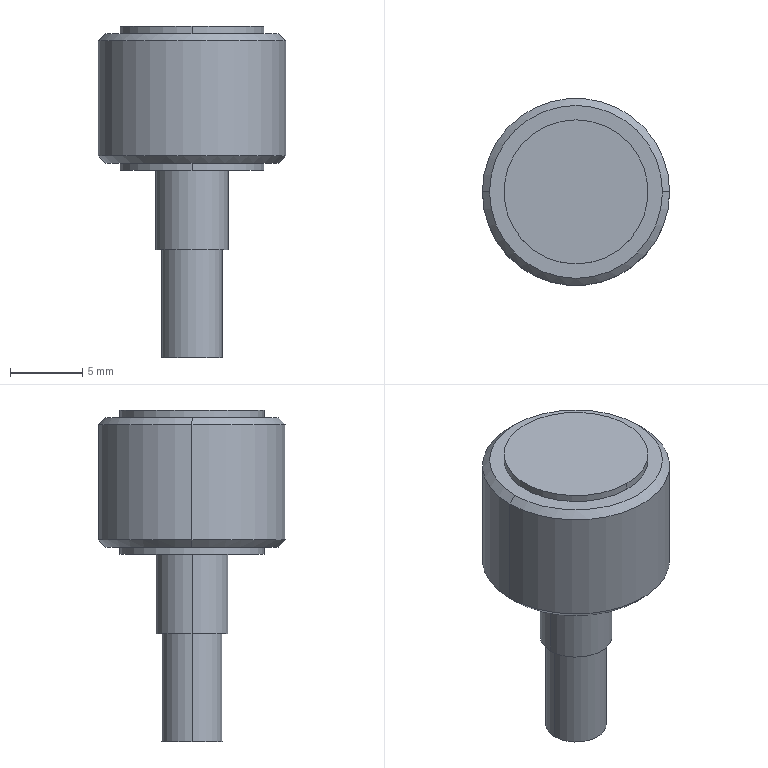Part | NX | 1 solid | 20 faces | box 13 x 13 x 23 mm | volume 1475 mm3 | cylinder 10 | plane 6 | cone 4 | commonest cylinder face diameters 10 x4 4.2 x2 5 x2 13 x2
STEP:
#1=CARTESIAN_POINT('',(0.,5.,0.));
#2=VERTEX_POINT('',#1);
#3=CARTESIAN_POINT('',(0.,-5.,0.));
#4=VERTEX_POINT('',#3);
#5=CARTESIAN_POINT('',(0.,0.,0.));
#6=DIRECTION('',(0.,0.,1.));
#7=DIRECTION('',(0.,-1.,0.));
#8=AXIS2_PLACEMENT_3D('',#5,#6,#7);
#9=CIRCLE('',#8,5.);
#10=EDGE_CURVE('',#2,#4,#9,.T.);
#11=ORIENTED_EDGE('',*,*,#10,.F.);
#12=CARTESIAN_POINT('',(0.,0.,0.));
#13=DIRECTION('',(0.,0.,1.));
#14=DIRECTION('',(0.,-1.,0.));
#15=AXIS2_PLACEMENT_3D('',#12,#13,#14);
#16=CIRCLE('',#15,5.);
#17=EDGE_CURVE('',#4,#2,#16,.T.);
#18=ORIENTED_EDGE('',*,*,#17,.F.);
#19=EDGE_LOOP('',(#11,#18));
#20=FACE_BOUND('',#19,.T.);
#21=CARTESIAN_POINT('',(2.5,0.,0.));
#22=VERTEX_POINT('',#21);
#23=CARTESIAN_POINT('',(-2.5,0.,0.));
#24=VERTEX_POINT('',#23);
#25=CARTESIAN_POINT('',(0.,0.,0.));
#26=DIRECTION('',(0.,0.,-1.));
#27=DIRECTION('',(1.,0.,0.));
#28=AXIS2_PLACEMENT_3D('',#25,#26,#27);
#29=CIRCLE('',#28,2.5);
#30=EDGE_CURVE('',#22,#24,#29,.T.);
#31=ORIENTED_EDGE('',*,*,#30,.F.);
#32=CARTESIAN_POINT('',(0.,0.,0.));
#33=DIRECTION('',(0.,0.,-1.));
#34=DIRECTION('',(1.,0.,0.));
#35=AXIS2_PLACEMENT_3D('',#32,#33,#34);
#36=CIRCLE('',#35,2.5);
#37=EDGE_CURVE('',#24,#22,#36,.T.);
#38=ORIENTED_EDGE('',*,*,#37,.F.);
#39=EDGE_LOOP('',(#31,#38));
#40=FACE_BOUND('',#39,.T.);
#41=CARTESIAN_POINT('',(0.,0.,0.));
#42=DIRECTION('',(0.,0.,1.));
#43=DIRECTION('',(1.,0.,0.));
#44=AXIS2_PLACEMENT_3D('',#41,#42,#43);
#45=PLANE('',#44);
#46=ADVANCED_FACE('',(#20,#40),#45,.F.);
#47=ORIENTED_EDGE('',*,*,#10,.T.);
#48=CARTESIAN_POINT('',(0.,-5.,0.5));
#49=VERTEX_POINT('',#48);
#50=CARTESIAN_POINT('',(0.,-5.,-0.5));
#51=DIRECTION('',(0.,0.,1.));
#52=VECTOR('',#51,1000.);
#53=LINE('',#50,#52);
#54=EDGE_CURVE('',#49,#4,#53,.F.);
#55=ORIENTED_EDGE('',*,*,#54,.F.);
#56=CARTESIAN_POINT('',(0.,5.,0.5));
#57=VERTEX_POINT('',#56);
#58=CARTESIAN_POINT('',(0.,0.,0.5));
#59=DIRECTION('',(0.,0.,-1.));
#60=DIRECTION('',(0.,1.,0.));
#61=AXIS2_PLACEMENT_3D('',#58,#59,#60);
#62=CIRCLE('',#61,5.);
#63=EDGE_CURVE('',#49,#57,#62,.T.);
#64=ORIENTED_EDGE('',*,*,#63,.T.);
#65=CARTESIAN_POINT('',(0.,5.,-0.5));
#66=DIRECTION('',(0.,0.,1.));
#67=VECTOR('',#66,1000.);
#68=LINE('',#65,#67);
#69=EDGE_CURVE('',#57,#2,#68,.F.);
#70=ORIENTED_EDGE('',*,*,#69,.T.);
#71=EDGE_LOOP('',(#47,#55,#64,#70));
#72=FACE_BOUND('',#71,.T.);
#73=CARTESIAN_POINT('',(0.,0.,-0.5));
#74=DIRECTION('',(0.,0.,1.));
#75=DIRECTION('',(0.,1.,0.));
#76=AXIS2_PLACEMENT_3D('',#73,#74,#75);
#77=CYLINDRICAL_SURFACE('',#76,5.);
#78=ADVANCED_FACE('',(#72),#77,.T.);
#79=CARTESIAN_POINT('',(-2.5,0.,-5.5));
#80=VERTEX_POINT('',#79);
#81=CARTESIAN_POINT('',(2.5,0.,-5.5));
#82=VERTEX_POINT('',#81);
#83=CARTESIAN_POINT('',(0.,0.,-5.5));
#84=DIRECTION('',(0.,0.,1.));
#85=DIRECTION('',(-1.,0.,0.));
#86=AXIS2_PLACEMENT_3D('',#83,#84,#85);
#87=CIRCLE('',#86,2.5);
#88=EDGE_CURVE('',#80,#82,#87,.T.);
#89=ORIENTED_EDGE('',*,*,#88,.T.);
#90=CARTESIAN_POINT('',(2.5,0.,0.));
#91=DIRECTION('',(0.,0.,-1.));
#92=VECTOR('',#91,1000.);
#93=LINE('',#90,#92);
#94=EDGE_CURVE('',#82,#22,#93,.F.);
#95=ORIENTED_EDGE('',*,*,#94,.T.);
#96=ORIENTED_EDGE('',*,*,#30,.T.);
#97=CARTESIAN_POINT('',(-2.5,0.,0.));
#98=DIRECTION('',(0.,0.,-1.));
#99=VECTOR('',#98,1000.);
#100=LINE('',#97,#99);
#101=EDGE_CURVE('',#80,#24,#100,.F.);
#102=ORIENTED_EDGE('',*,*,#101,.F.);
#103=EDGE_LOOP('',(#89,#95,#96,#102));
#104=FACE_BOUND('',#103,.T.);
#105=CARTESIAN_POINT('',(0.,0.,0.));
#106=DIRECTION('',(0.,0.,-1.));
#107=DIRECTION('',(-1.,0.,0.));
#108=AXIS2_PLACEMENT_3D('',#105,#106,#107);
#109=CYLINDRICAL_SURFACE('',#108,2.5);
#110=ADVANCED_FACE('',(#104),#109,.T.);
#111=CARTESIAN_POINT('',(-6.,0.,0.5));
#112=VERTEX_POINT('',#111);
#113=CARTESIAN_POINT('',(6.,0.,0.5));
#114=VERTEX_POINT('',#113);
#115=CARTESIAN_POINT('',(0.,0.,0.5));
#116=DIRECTION('',(0.,0.,1.));
#117=DIRECTION('',(-1.,0.,0.));
#118=AXIS2_PLACEMENT_3D('',#115,#116,#117);
#119=CIRCLE('',#118,6.);
#120=EDGE_CURVE('',#112,#114,#119,.T.);
#121=ORIENTED_EDGE('',*,*,#120,.F.);
#122=CARTESIAN_POINT('',(0.,0.,0.5));
#123=DIRECTION('',(0.,0.,1.));
#124=DIRECTION('',(-1.,0.,0.));
#125=AXIS2_PLACEMENT_3D('',#122,#123,#124);
#126=CIRCLE('',#125,6.);
#127=EDGE_CURVE('',#114,#112,#126,.T.);
#128=ORIENTED_EDGE('',*,*,#127,.F.);
#129=EDGE_LOOP('',(#121,#128));
#130=FACE_BOUND('',#129,.T.);
#131=CARTESIAN_POINT('',(0.,0.,0.5));
#132=DIRECTION('',(0.,0.,-1.));
#133=DIRECTION('',(0.,1.,0.));
#134=AXIS2_PLACEMENT_3D('',#131,#132,#133);
#135=CIRCLE('',#134,5.);
#136=EDGE_CURVE('',#57,#49,#135,.T.);
#137=ORIENTED_EDGE('',*,*,#136,.F.);
#138=ORIENTED_EDGE('',*,*,#63,.F.);
#139=EDGE_LOOP('',(#137,#138));
#140=FACE_BOUND('',#139,.T.);
#141=CARTESIAN_POINT('',(0.,0.,0.5));
#142=DIRECTION('',(0.,0.,1.));
#143=DIRECTION('',(1.,0.,0.));
#144=AXIS2_PLACEMENT_3D('',#141,#142,#143);
#145=PLANE('',#144);
#146=ADVANCED_FACE('',(#130,#140),#145,.F.);
#147=ORIENTED_EDGE('',*,*,#120,.T.);
#148=CARTESIAN_POINT('',(6.5,0.,1.));
#149=VERTEX_POINT('',#148);
#150=CARTESIAN_POINT('',(6.25,0.,0.75));
#151=DIRECTION('',(0.7071,0.,0.7071));
#152=VECTOR('',#151,1000.);
#153=LINE('',#150,#152);
#154=EDGE_CURVE('',#114,#149,#153,.T.);
#155=ORIENTED_EDGE('',*,*,#154,.T.);
#156=CARTESIAN_POINT('',(-6.5,0.,1.));
#157=VERTEX_POINT('',#156);
#158=CARTESIAN_POINT('',(0.,0.,1.));
#159=DIRECTION('',(0.,0.,1.));
#160=DIRECTION('',(-1.,0.,0.));
#161=AXIS2_PLACEMENT_3D('',#158,#159,#160);
#162=CIRCLE('',#161,6.5);
#163=EDGE_CURVE('',#157,#149,#162,.T.);
#164=ORIENTED_EDGE('',*,*,#163,.F.);
#165=CARTESIAN_POINT('',(-6.25,0.,0.75));
#166=DIRECTION('',(-0.7071,0.,0.7071));
#167=VECTOR('',#166,1000.);
#168=LINE('',#165,#167);
#169=EDGE_CURVE('',#112,#157,#168,.T.);
#170=ORIENTED_EDGE('',*,*,#169,.F.);
#171=EDGE_LOOP('',(#147,#155,#164,#170));
#172=FACE_BOUND('',#171,.T.);
#173=CARTESIAN_POINT('',(0.,0.,0.75));
#174=DIRECTION('',(0.,0.,1.));
#175=DIRECTION('',(1.,0.,0.));
#176=AXIS2_PLACEMENT_3D('',#173,#174,#175);
#177=CONICAL_SURFACE('',#176,6.25,0.7854);
#178=ADVANCED_FACE('',(#172),#177,.T.);
#179=CARTESIAN_POINT('',(6.5,0.,9.));
#180=VERTEX_POINT('',#179);
#181=CARTESIAN_POINT('',(-6.5,0.,9.));
#182=VERTEX_POINT('',#181);
#183=CARTESIAN_POINT('',(0.,0.,9.));
#184=DIRECTION('',(0.,0.,-1.));
#185=DIRECTION('',(1.,0.,0.));
#186=AXIS2_PLACEMENT_3D('',#183,#184,#185);
#187=CIRCLE('',#186,6.5);
#188=EDGE_CURVE('',#180,#182,#187,.T.);
#189=ORIENTED_EDGE('',*,*,#188,.T.);
#190=CARTESIAN_POINT('',(-6.5,0.,0.));
#191=DIRECTION('',(0.,0.,1.));
#192=VECTOR('',#191,1000.);
#193=LINE('',#190,#192);
#194=EDGE_CURVE('',#182,#157,#193,.F.);
#195=ORIENTED_EDGE('',*,*,#194,.T.);
#196=ORIENTED_EDGE('',*,*,#163,.T.);
#197=CARTESIAN_POINT('',(6.5,0.,0.));
#198=DIRECTION('',(0.,0.,1.));
#199=VECTOR('',#198,1000.);
#200=LINE('',#197,#199);
#201=EDGE_CURVE('',#180,#149,#200,.F.);
#202=ORIENTED_EDGE('',*,*,#201,.F.);
#203=EDGE_LOOP('',(#189,#195,#196,#202));
#204=FACE_BOUND('',#203,.T.);
#205=CARTESIAN_POINT('',(0.,0.,0.));
#206=DIRECTION('',(0.,0.,1.));
#207=DIRECTION('',(1.,0.,0.));
#208=AXIS2_PLACEMENT_3D('',#205,#206,#207);
#209=CYLINDRICAL_SURFACE('',#208,6.5);
#210=ADVANCED_FACE('',(#204),#209,.T.);
#211=ORIENTED_EDGE('',*,*,#188,.F.);
#212=CARTESIAN_POINT('',(6.,0.,9.5));
#213=VERTEX_POINT('',#212);
#214=CARTESIAN_POINT('',(6.25,0.,9.25));
#215=DIRECTION('',(0.7071,0.,-0.7071));
#216=VECTOR('',#215,1000.);
#217=LINE('',#214,#216);
#218=EDGE_CURVE('',#213,#180,#217,.T.);
#219=ORIENTED_EDGE('',*,*,#218,.F.);
#220=CARTESIAN_POINT('',(-6.,0.,9.5));
#221=VERTEX_POINT('',#220);
#222=CARTESIAN_POINT('',(0.,0.,9.5));
#223=DIRECTION('',(0.,0.,-1.));
#224=DIRECTION('',(1.,0.,0.));
#225=AXIS2_PLACEMENT_3D('',#222,#223,#224);
#226=CIRCLE('',#225,6.);
#227=EDGE_CURVE('',#213,#221,#226,.T.);
#228=ORIENTED_EDGE('',*,*,#227,.T.);
#229=CARTESIAN_POINT('',(-6.25,0.,9.25));
#230=DIRECTION('',(-0.7071,0.,-0.7071));
#231=VECTOR('',#230,1000.);
#232=LINE('',#229,#231);
#233=EDGE_CURVE('',#221,#182,#232,.T.);
#234=ORIENTED_EDGE('',*,*,#233,.T.);
#235=EDGE_LOOP('',(#211,#219,#228,#234));
#236=FACE_BOUND('',#235,.T.);
#237=CARTESIAN_POINT('',(0.,0.,9.25));
#238=DIRECTION('',(0.,0.,-1.));
#239=DIRECTION('',(-1.,0.,0.));
#240=AXIS2_PLACEMENT_3D('',#237,#238,#239);
#241=CONICAL_SURFACE('',#240,6.25,0.7854);
#242=ADVANCED_FACE('',(#236),#241,.T.);
#243=CARTESIAN_POINT('',(2.1,0.,-13.));
#244=VERTEX_POINT('',#243);
#245=CARTESIAN_POINT('',(-2.1,0.,-13.));
#246=VERTEX_POINT('',#245);
#247=CARTESIAN_POINT('',(0.,0.,-13.));
#248=DIRECTION('',(0.,0.,1.));
#249=DIRECTION('',(1.,0.,0.));
#250=AXIS2_PLACEMENT_3D('',#247,#248,#249);
#251=CIRCLE('',#250,2.1);
#252=EDGE_CURVE('',#244,#246,#251,.T.);
#253=ORIENTED_EDGE('',*,*,#252,.T.);
#254=CARTESIAN_POINT('',(-2.1,0.,-5.5));
#255=VERTEX_POINT('',#254);
#256=CARTESIAN_POINT('',(-2.1,0.,-5.5));
#257=DIRECTION('',(0.,0.,-1.));
#258=VECTOR('',#257,1000.);
#259=LINE('',#256,#258);
#260=EDGE_CURVE('',#246,#255,#259,.F.);
#261=ORIENTED_EDGE('',*,*,#260,.T.);
#262=CARTESIAN_POINT('',(2.1,0.,-5.5));
#263=VERTEX_POINT('',#262);
#264=CARTESIAN_POINT('',(0.,0.,-5.5));
#265=DIRECTION('',(0.,0.,-1.));
#266=DIRECTION('',(1.,0.,0.));
#267=AXIS2_PLACEMENT_3D('',#264,#265,#266);
#268=CIRCLE('',#267,2.1);
#269=EDGE_CURVE('',#255,#263,#268,.T.);
#270=ORIENTED_EDGE('',*,*,#269,.T.);
#271=CARTESIAN_POINT('',(2.1,0.,-5.5));
#272=DIRECTION('',(0.,0.,-1.));
#273=VECTOR('',#272,1000.);
#274=LINE('',#271,#273);
#275=EDGE_CURVE('',#244,#263,#274,.F.);
#276=ORIENTED_EDGE('',*,*,#275,.F.);
#277=EDGE_LOOP('',(#253,#261,#270,#276));
#278=FACE_BOUND('',#277,.T.);
#279=CARTESIAN_POINT('',(0.,0.,-5.5));
#280=DIRECTION('',(0.,0.,-1.));
#281=DIRECTION('',(-1.,0.,0.));
#282=AXIS2_PLACEMENT_3D('',#279,#280,#281);
#283=CYLINDRICAL_SURFACE('',#282,2.1);
#284=ADVANCED_FACE('',(#278),#283,.T.);
#285=ORIENTED_EDGE('',*,*,#88,.F.);
#286=CARTESIAN_POINT('',(0.,0.,-5.5));
#287=DIRECTION('',(0.,0.,1.));
#288=DIRECTION('',(-1.,0.,0.));
#289=AXIS2_PLACEMENT_3D('',#286,#287,#288);
#290=CIRCLE('',#289,2.5);
#291=EDGE_CURVE('',#82,#80,#290,.T.);
#292=ORIENTED_EDGE('',*,*,#291,.F.);
#293=EDGE_LOOP('',(#285,#292));
#294=FACE_BOUND('',#293,.T.);
#295=ORIENTED_EDGE('',*,*,#269,.F.);
#296=CARTESIAN_POINT('',(0.,0.,-5.5));
#297=DIRECTION('',(0.,0.,-1.));
#298=DIRECTION('',(1.,0.,0.));
#299=AXIS2_PLACEMENT_3D('',#296,#297,#298);
#300=CIRCLE('',#299,2.1);
#301=EDGE_CURVE('',#263,#255,#300,.T.);
#302=ORIENTED_EDGE('',*,*,#301,.F.);
#303=EDGE_LOOP('',(#295,#302));
#304=FACE_BOUND('',#303,.T.);
#305=CARTESIAN_POINT('',(0.,0.,-5.5));
#306=DIRECTION('',(0.,0.,-1.));
#307=DIRECTION('',(0.,-1.,0.));
#308=AXIS2_PLACEMENT_3D('',#305,#306,#307);
#309=PLANE('',#308);
#310=ADVANCED_FACE('',(#294,#304),#309,.T.);
#311=ORIENTED_EDGE('',*,*,#252,.F.);
#312=CARTESIAN_POINT('',(0.,0.,-13.));
#313=DIRECTION('',(0.,0.,1.));
#314=DIRECTION('',(1.,0.,0.));
#315=AXIS2_PLACEMENT_3D('',#312,#313,#314);
#316=CIRCLE('',#315,2.1);
#317=EDGE_CURVE('',#246,#244,#316,.T.);
#318=ORIENTED_EDGE('',*,*,#317,.F.);
#319=EDGE_LOOP('',(#311,#318));
#320=FACE_BOUND('',#319,.T.);
#321=CARTESIAN_POINT('',(0.,0.,-13.));
#322=DIRECTION('',(0.,0.,-1.));
#323=DIRECTION('',(0.,-1.,0.));
#324=AXIS2_PLACEMENT_3D('',#321,#322,#323);
#325=PLANE('',#324);
#326=ADVANCED_FACE('',(#320),#325,.T.);
#327=CARTESIAN_POINT('',(0.,0.,9.5));
#328=DIRECTION('',(0.,0.,-1.));
#329=DIRECTION('',(1.,0.,0.));
#330=AXIS2_PLACEMENT_3D('',#327,#328,#329);
#331=CIRCLE('',#330,6.);
#332=EDGE_CURVE('',#221,#213,#331,.T.);
#333=ORIENTED_EDGE('',*,*,#332,.F.);
#334=ORIENTED_EDGE('',*,*,#227,.F.);
#335=EDGE_LOOP('',(#333,#334));
#336=FACE_BOUND('',#335,.T.);
#337=CARTESIAN_POINT('',(0.,5.,9.5));
#338=VERTEX_POINT('',#337);
#339=CARTESIAN_POINT('',(0.,-5.,9.5));
#340=VERTEX_POINT('',#339);
#341=CARTESIAN_POINT('',(0.,0.,9.5));
#342=DIRECTION('',(0.,0.,1.));
#343=DIRECTION('',(0.,-1.,0.));
#344=AXIS2_PLACEMENT_3D('',#341,#342,#343);
#345=CIRCLE('',#344,5.);
#346=EDGE_CURVE('',#338,#340,#345,.T.);
#347=ORIENTED_EDGE('',*,*,#346,.F.);
#348=CARTESIAN_POINT('',(0.,0.,9.5));
#349=DIRECTION('',(0.,0.,1.));
#350=DIRECTION('',(0.,-1.,0.));
#351=AXIS2_PLACEMENT_3D('',#348,#349,#350);
#352=CIRCLE('',#351,5.);
#353=EDGE_CURVE('',#340,#338,#352,.T.);
#354=ORIENTED_EDGE('',*,*,#353,.F.);
#355=EDGE_LOOP('',(#347,#354));
#356=FACE_BOUND('',#355,.T.);
#357=CARTESIAN_POINT('',(0.,0.,9.5));
#358=DIRECTION('',(0.,0.,1.));
#359=DIRECTION('',(1.,0.,0.));
#360=AXIS2_PLACEMENT_3D('',#357,#358,#359);
#361=PLANE('',#360);
#362=ADVANCED_FACE('',(#336,#356),#361,.T.);
#363=CARTESIAN_POINT('',(0.,5.,10.));
#364=VERTEX_POINT('',#363);
#365=CARTESIAN_POINT('',(0.,-5.,10.));
#366=VERTEX_POINT('',#365);
#367=CARTESIAN_POINT('',(0.,0.,10.));
#368=DIRECTION('',(0.,0.,-1.));
#369=DIRECTION('',(0.,1.,0.));
#370=AXIS2_PLACEMENT_3D('',#367,#368,#369);
#371=CIRCLE('',#370,5.);
#372=EDGE_CURVE('',#364,#366,#371,.T.);
#373=ORIENTED_EDGE('',*,*,#372,.T.);
#374=CARTESIAN_POINT('',(0.,-5.,-0.5));
#375=DIRECTION('',(0.,0.,1.));
#376=VECTOR('',#375,1000.);
#377=LINE('',#374,#376);
#378=EDGE_CURVE('',#366,#340,#377,.F.);
#379=ORIENTED_EDGE('',*,*,#378,.T.);
#380=ORIENTED_EDGE('',*,*,#353,.T.);
#381=CARTESIAN_POINT('',(0.,5.,-0.5));
#382=DIRECTION('',(0.,0.,1.));
#383=VECTOR('',#382,1000.);
#384=LINE('',#381,#383);
#385=EDGE_CURVE('',#364,#338,#384,.F.);
#386=ORIENTED_EDGE('',*,*,#385,.F.);
#387=EDGE_LOOP('',(#373,#379,#380,#386));
#388=FACE_BOUND('',#387,.T.);
#389=CARTESIAN_POINT('',(0.,0.,-0.5));
#390=DIRECTION('',(0.,0.,1.));
#391=DIRECTION('',(0.,1.,0.));
#392=AXIS2_PLACEMENT_3D('',#389,#390,#391);
#393=CYLINDRICAL_SURFACE('',#392,5.);
#394=ADVANCED_FACE('',(#388),#393,.T.);
#395=ORIENTED_EDGE('',*,*,#372,.F.);
#396=CARTESIAN_POINT('',(0.,0.,10.));
#397=DIRECTION('',(0.,0.,-1.));
#398=DIRECTION('',(0.,1.,0.));
#399=AXIS2_PLACEMENT_3D('',#396,#397,#398);
#400=CIRCLE('',#399,5.);
#401=EDGE_CURVE('',#366,#364,#400,.T.);
#402=ORIENTED_EDGE('',*,*,#401,.F.);
#403=EDGE_LOOP('',(#395,#402));
#404=FACE_BOUND('',#403,.T.);
#405=CARTESIAN_POINT('',(0.,0.,10.));
#406=DIRECTION('',(0.,0.,1.));
#407=DIRECTION('',(1.,0.,0.));
#408=AXIS2_PLACEMENT_3D('',#405,#406,#407);
#409=PLANE('',#408);
#410=ADVANCED_FACE('',(#404),#409,.T.);
#411=ORIENTED_EDGE('',*,*,#332,.T.);
#412=ORIENTED_EDGE('',*,*,#218,.T.);
#413=CARTESIAN_POINT('',(0.,0.,9.));
#414=DIRECTION('',(0.,0.,-1.));
#415=DIRECTION('',(1.,0.,0.));
#416=AXIS2_PLACEMENT_3D('',#413,#414,#415);
#417=CIRCLE('',#416,6.5);
#418=EDGE_CURVE('',#182,#180,#417,.T.);
#419=ORIENTED_EDGE('',*,*,#418,.F.);
#420=ORIENTED_EDGE('',*,*,#233,.F.);
#421=EDGE_LOOP('',(#411,#412,#419,#420));
#422=FACE_BOUND('',#421,.T.);
#423=CARTESIAN_POINT('',(0.,0.,9.25));
#424=DIRECTION('',(0.,0.,-1.));
#425=DIRECTION('',(-1.,0.,0.));
#426=AXIS2_PLACEMENT_3D('',#423,#424,#425);
#427=CONICAL_SURFACE('',#426,6.25,0.7854);
#428=ADVANCED_FACE('',(#422),#427,.T.);
#429=ORIENTED_EDGE('',*,*,#260,.F.);
#430=ORIENTED_EDGE('',*,*,#317,.T.);
#431=ORIENTED_EDGE('',*,*,#275,.T.);
#432=ORIENTED_EDGE('',*,*,#301,.T.);
#433=EDGE_LOOP('',(#429,#430,#431,#432));
#434=FACE_BOUND('',#433,.T.);
#435=CARTESIAN_POINT('',(0.,0.,-5.5));
#436=DIRECTION('',(0.,0.,-1.));
#437=DIRECTION('',(-1.,0.,0.));
#438=AXIS2_PLACEMENT_3D('',#435,#436,#437);
#439=CYLINDRICAL_SURFACE('',#438,2.1);
#440=ADVANCED_FACE('',(#434),#439,.T.);
#441=CARTESIAN_POINT('',(0.,0.,1.));
#442=DIRECTION('',(0.,0.,1.));
#443=DIRECTION('',(-1.,0.,0.));
#444=AXIS2_PLACEMENT_3D('',#441,#442,#443);
#445=CIRCLE('',#444,6.5);
#446=EDGE_CURVE('',#149,#157,#445,.T.);
#447=ORIENTED_EDGE('',*,*,#446,.T.);
#448=ORIENTED_EDGE('',*,*,#194,.F.);
#449=ORIENTED_EDGE('',*,*,#418,.T.);
#450=ORIENTED_EDGE('',*,*,#201,.T.);
#451=EDGE_LOOP('',(#447,#448,#449,#450));
#452=FACE_BOUND('',#451,.T.);
#453=CARTESIAN_POINT('',(0.,0.,0.));
#454=DIRECTION('',(0.,0.,1.));
#455=DIRECTION('',(1.,0.,0.));
#456=AXIS2_PLACEMENT_3D('',#453,#454,#455);
#457=CYLINDRICAL_SURFACE('',#456,6.5);
#458=ADVANCED_FACE('',(#452),#457,.T.);
#459=ORIENTED_EDGE('',*,*,#446,.F.);
#460=ORIENTED_EDGE('',*,*,#154,.F.);
#461=ORIENTED_EDGE('',*,*,#127,.T.);
#462=ORIENTED_EDGE('',*,*,#169,.T.);
#463=EDGE_LOOP('',(#459,#460,#461,#462));
#464=FACE_BOUND('',#463,.T.);
#465=CARTESIAN_POINT('',(0.,0.,0.75));
#466=DIRECTION('',(0.,0.,1.));
#467=DIRECTION('',(1.,0.,0.));
#468=AXIS2_PLACEMENT_3D('',#465,#466,#467);
#469=CONICAL_SURFACE('',#468,6.25,0.7854);
#470=ADVANCED_FACE('',(#464),#469,.T.);
#471=ORIENTED_EDGE('',*,*,#101,.T.);
#472=ORIENTED_EDGE('',*,*,#37,.T.);
#473=ORIENTED_EDGE('',*,*,#94,.F.);
#474=ORIENTED_EDGE('',*,*,#291,.T.);
#475=EDGE_LOOP('',(#471,#472,#473,#474));
#476=FACE_BOUND('',#475,.T.);
#477=CARTESIAN_POINT('',(0.,0.,0.));
#478=DIRECTION('',(0.,0.,-1.));
#479=DIRECTION('',(-1.,0.,0.));
#480=AXIS2_PLACEMENT_3D('',#477,#478,#479);
#481=CYLINDRICAL_SURFACE('',#480,2.5);
#482=ADVANCED_FACE('',(#476),#481,.T.);
#483=ORIENTED_EDGE('',*,*,#136,.T.);
#484=ORIENTED_EDGE('',*,*,#54,.T.);
#485=ORIENTED_EDGE('',*,*,#17,.T.);
#486=ORIENTED_EDGE('',*,*,#69,.F.);
#487=EDGE_LOOP('',(#483,#484,#485,#486));
#488=FACE_BOUND('',#487,.T.);
#489=CARTESIAN_POINT('',(0.,0.,-0.5));
#490=DIRECTION('',(0.,0.,1.));
#491=DIRECTION('',(0.,1.,0.));
#492=AXIS2_PLACEMENT_3D('',#489,#490,#491);
#493=CYLINDRICAL_SURFACE('',#492,5.);
#494=ADVANCED_FACE('',(#488),#493,.T.);
#495=ORIENTED_EDGE('',*,*,#346,.T.);
#496=ORIENTED_EDGE('',*,*,#378,.F.);
#497=ORIENTED_EDGE('',*,*,#401,.T.);
#498=ORIENTED_EDGE('',*,*,#385,.T.);
#499=EDGE_LOOP('',(#495,#496,#497,#498));
#500=FACE_BOUND('',#499,.T.);
#501=CARTESIAN_POINT('',(0.,0.,-0.5));
#502=DIRECTION('',(0.,0.,1.));
#503=DIRECTION('',(0.,1.,0.));
#504=AXIS2_PLACEMENT_3D('',#501,#502,#503);
#505=CYLINDRICAL_SURFACE('',#504,5.);
#506=ADVANCED_FACE('',(#500),#505,.T.);
#507=CLOSED_SHELL('',(#46,#78,#110,#146,#178,#210,#242,#284,#310,#326,#362,#394,#410,#428,#440,#458,#470,#482,#494,#506));
#508=MANIFOLD_SOLID_BREP('',#507);
#509=(LENGTH_UNIT()NAMED_UNIT(*)SI_UNIT(.MILLI.,.METRE.));
#510=UNCERTAINTY_MEASURE_WITH_UNIT(LENGTH_MEASURE(0.00001),#509,'','');
#511=(NAMED_UNIT(*)PLANE_ANGLE_UNIT()SI_UNIT($,.RADIAN.));
#512=(NAMED_UNIT(*)SI_UNIT($,.STERADIAN.)SOLID_ANGLE_UNIT());
#513=(GEOMETRIC_REPRESENTATION_CONTEXT(3)GLOBAL_UNCERTAINTY_ASSIGNED_CONTEXT((#510))GLOBAL_UNIT_ASSIGNED_CONTEXT((#509,#511,#512))REPRESENTATION_CONTEXT('',''));
#514=ADVANCED_BREP_SHAPE_REPRESENTATION('',(#508),#513);